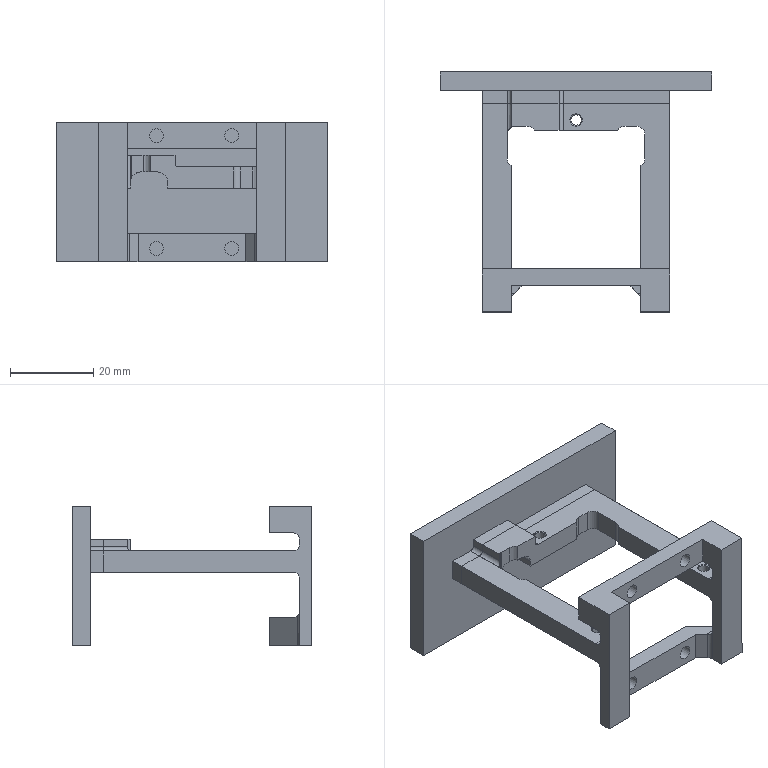NC program | NX | posted with a generic post | part box 65 x 57.5 x 33.5 mm
Whole program:
N10 G17 G21 G94 G90
(PLANAR_PROFILING , TOOL : D8-25-D8-60-3T-ROUGH)
N12 T02 M6
N14 G54
N16 G17 G0 G90 X-10. Y-1.1 B0. C0. S4500 M3
N18 G43 Z37. H2
N20 Z8.507 B-180.
N22 G94 G1 Z6.507 F1500.
N24 X0.
N26 X45.
N28 X55.
N30 Z8.507
N32 G0 Z8.014
N34 G1 Z6.014
N36 X45.
N38 X0.
N40 X-10.
N42 Z8.014
N44 G0 Z7.521
N46 G1 Z5.521
N48 X0.
N50 X45.
N52 X55.
N54 Z7.521
N56 G0 Z7.029
N58 G1 Z5.029
N60 X45.
N62 X0.
N64 X-10.
N66 Z7.029
N68 G0 Z6.536
N70 G1 Z4.536
N72 X0.
N74 X45.
N76 X55.
N78 Z6.536
N80 G0 Z6.043
N82 G1 Z4.043
N84 X45.
N86 X0.
N88 X-10.
N90 Z6.043
N92 G0 Z5.55
N94 G1 Z3.55
N96 X0.
N98 X45.
N100 X55.
N102 Z5.55
N104 G0 Z5.057
N106 G1 Z3.057
N108 X45.
N110 X0.
N112 X-10.
N114 Z5.057
N116 G0 Z4.564
N118 G1 Z2.564
N120 X0.
N122 X45.
N124 X55.
N126 Z4.564
N128 G0 Z4.071
N130 G1 Z2.071
N132 X45.
N134 X0.
N136 X-10.
N138 Z4.071
N140 G0 Z3.579
N142 G1 Z1.579
N144 X0.
N146 X45.
N148 X55.
N150 Z3.579
N152 G0 Z3.086
N154 G1 Z1.086
N156 X45.
N158 X0.
N160 X-10.
N162 Z3.086
N164 G0 Z2.593
N166 G1 Z0.593
N168 X0.
N170 X45.
N172 X55.
N174 Z2.593
N176 G0 Z2.1
N178 G1 Z0.1
N180 X45.
N182 X0.
N184 X-10.
N186 Z2.1
N188 G0 Z37.
N190 M5
(PLANAR_PROFILING_COPY , TOOL : D8-25-D8-60-3T-FINISH)
N192 T03 M6
N194 G54
N196 G17 G0 G90 X-10. Y-1.1 B0. C0. S4500 M3
N198 G43 Z37. H3
N200 Z2. B-180.
N202 G94 G1 Z0. F1000.
N204 X0.
N206 X45.
N208 X55.
N210 Z2.
N212 G0 Z37.
N214 M5
(PLANAR_PROFILING_1 , TOOL : D3-9-D4-50-3T-ROUGH)
N216 T05 M6
N218 G54
N220 G17 G0 G90 X23.07 Y5.785 B0. C0. S4500 M3
N222 G43 Z30. H5
N224 Z2.708 B-180.
N226 G94 G1 Z-0.292 F1500.
N228 Y3.1
N230 G3 X24.57 Y1.6 R1.5
N232 G1 X24.97
N234 Y2.8
N236 G2 X26.57 Y4.4 R1.6
N238 G1 X38.
N240 G2 X39.6 Y2.8 R1.6
N242 G1 Y1.6
N244 X40.
N246 G3 X41.5 Y3.1 R1.5
N248 G1 Y5.785
N250 Z2.708
N252 G0 Z2.417
N254 G1 Z-0.583
N256 Y3.1
N258 G2 X40. Y1.6 R1.5
N260 G1 X39.6
N262 Y2.8
N264 G3 X38. Y4.4 R1.6
N266 G1 X26.57
N268 G3 X24.97 Y2.8 R1.6
N270 G1 Y1.6
N272 X24.57
N274 G2 X23.07 Y3.1 R1.5
N276 G1 Y5.785
N278 Z2.417
N280 G0 Z2.125
N282 G1 Z-0.875
N284 Y3.1
N286 G3 X24.57 Y1.6 R1.5
N288 G1 X24.97
N290 Y2.8
N292 G2 X26.57 Y4.4 R1.6
N294 G1 X38.
N296 G2 X39.6 Y2.8 R1.6
N298 G1 Y1.6
N300 X40.
N302 G3 X41.5 Y3.1 R1.5
N304 G1 Y5.785
N306 Z2.125
N308 G0 Z1.833
N310 G1 Z-1.167
N312 Y3.1
N314 G2 X40. Y1.6 R1.5
N316 G1 X39.6
N318 Y2.8
N320 G3 X38. Y4.4 R1.6
N322 G1 X26.57
N324 G3 X24.97 Y2.8 R1.6
N326 G1 Y1.6
N328 X24.57
N330 G2 X23.07 Y3.1 R1.5
N332 G1 Y5.785
N334 Z1.833
N336 G0 Z1.542
N338 G1 Z-1.458
N340 Y3.1
N342 G3 X24.57 Y1.6 R1.5
N344 G1 X24.97
N346 Y2.8
N348 G2 X26.57 Y4.4 R1.6
N350 G1 X38.
N352 G2 X39.6 Y2.8 R1.6
N354 G1 Y1.6
N356 X40.
N358 G3 X41.5 Y3.1 R1.5
N360 G1 Y5.785
N362 Z1.542
N364 G0 Z1.25
N366 G1 Z-1.75
N368 Y3.1
N370 G2 X40. Y1.6 R1.5
N372 G1 X39.6
N374 Y2.8
N376 G3 X38. Y4.4 R1.6
N378 G1 X26.57
N380 G3 X24.97 Y2.8 R1.6
N382 G1 Y1.6
N384 X24.57
N386 G2 X23.07 Y3.1 R1.5
N388 G1 Y5.785
N390 Z1.25
N392 G0 Z0.958
N394 G1 Z-2.042
N396 Y3.1
N398 G3 X24.57 Y1.6 R1.5
N400 G1 X24.97
N402 Y2.8
N404 G2 X26.57 Y4.4 R1.6
N406 G1 X38.
N408 G2 X39.6 Y2.8 R1.6
N410 G1 Y1.6
N412 X40.
N414 G3 X41.5 Y3.1 R1.5
N416 G1 Y5.785
N418 Z0.958
N420 G0 Z0.667
N422 G1 Z-2.333
N424 Y3.1
N426 G2 X40. Y1.6 R1.5
N428 G1 X39.6
N430 Y2.8
N432 G3 X38. Y4.4 R1.6
N434 G1 X26.57
N436 G3 X24.97 Y2.8 R1.6
N438 G1 Y1.6
N440 X24.57
N442 G2 X23.07 Y3.1 R1.5
N444 G1 Y5.785
N446 Z0.667
N448 G0 Z0.375
N450 G1 Z-2.625
N452 Y3.1
N454 G3 X24.57 Y1.6 R1.5
N456 G1 X24.97
N458 Y2.8
N460 G2 X26.57 Y4.4 R1.6
N462 G1 X38.
N464 G2 X39.6 Y2.8 R1.6
N466 G1 Y1.6
N468 X40.
N470 G3 X41.5 Y3.1 R1.5
N472 G1 Y5.785
N474 Z0.375
N476 G0 Z0.083
N478 G1 Z-2.917
N480 Y3.1
N482 G2 X40. Y1.6 R1.5
N484 G1 X39.6
N486 Y2.8
N488 G3 X38. Y4.4 R1.6
N490 G1 X26.57
N492 G3 X24.97 Y2.8 R1.6
N494 G1 Y1.6
N496 X24.57
N498 G2 X23.07 Y3.1 R1.5
N500 G1 Y5.785
N502 Z0.083
N504 G0 Z-0.208
N506 G1 Z-3.208
N508 Y3.1
N510 G3 X24.57 Y1.6 R1.5
N512 G1 X24.97
N514 Y2.8
N516 G2 X26.57 Y4.4 R1.6
N518 G1 X38.
N520 G2 X39.6 Y2.8 R1.6
N522 G1 Y1.6
N524 X40.
N526 G3 X41.5 Y3.1 R1.5
N528 G1 Y5.785
N530 Z-0.208
N532 G0 Z-0.5
N534 G1 Z-3.5
N536 Y3.1
N538 G2 X40. Y1.6 R1.5
N540 G1 X39.6
N542 Y2.8
N544 G3 X38. Y4.4 R1.6
N546 G1 X26.57
N548 G3 X24.97 Y2.8 R1.6
N550 G1 Y1.6
N552 X24.57
N554 G2 X23.07 Y3.1 R1.5
N556 G1 Y5.785
N558 Z-0.5
N560 G0 Z-0.792
N562 G1 Z-3.792
N564 Y3.1
N566 G3 X24.57 Y1.6 R1.5
N568 G1 X24.97
N570 Y2.8
N572 G2 X26.57 Y4.4 R1.6
N574 G1 X38.
N576 G2 X39.6 Y2.8 R1.6
N578 G1 Y1.6
N580 X40.
N582 G3 X41.5 Y3.1 R1.5
N584 G1 Y5.785
N586 Z-0.792
N588 G0 Z-1.083
N590 G1 Z-4.083
N592 Y3.1
N594 G2 X40. Y1.6 R1.5
N596 G1 X39.6
N598 Y2.8
N600 G3 X38. Y4.4 R1.6
N602 G1 X26.57
N604 G3 X24.97 Y2.8 R1.6
N606 G1 Y1.6
N608 X24.57
N610 G2 X23.07 Y3.1 R1.5
N612 G1 Y5.785
N614 Z-1.083
N616 G0 Z-1.375
N618 G1 Z-4.375
N620 Y3.1
N622 G3 X24.57 Y1.6 R1.5
N624 G1 X24.97
N626 Y2.8
N628 G2 X26.57 Y4.4 R1.6
N630 G1 X38.
N632 G2 X39.6 Y2.8 R1.6
N634 G1 Y1.6
N636 X40.
N638 G3 X41.5 Y3.1 R1.5
N640 G1 Y5.785
N642 Z-1.375
N644 G0 Z-1.667
N646 G1 Z-4.667
N648 Y3.1
N650 G2 X40. Y1.6 R1.5
N652 G1 X39.6
N654 Y2.8
N656 G3 X38. Y4.4 R1.6
N658 G1 X26.57
N660 G3 X24.97 Y2.8 R1.6
N662 G1 Y1.6
N664 X24.57
N666 G2 X23.07 Y3.1 R1.5
N668 G1 Y5.785
N670 Z-1.667
N672 G0 Z-1.958
N674 G1 Z-4.958
N676 Y3.1
N678 G3 X24.57 Y1.6 R1.5
N680 G1 X24.97
N682 Y2.8
N684 G2 X26.57 Y4.4 R1.6
N686 G1 X38.
N688 G2 X39.6 Y2.8 R1.6
N690 G1 Y1.6
N692 X40.
N694 G3 X41.5 Y3.1 R1.5
N696 G1 Y5.785
N698 Z-1.958
N700 G0 Z-2.25
N702 G1 Z-5.25
N704 Y3.1
N706 G2 X40. Y1.6 R1.5
N708 G1 X39.6
N710 Y2.8
N712 G3 X38. Y4.4 R1.6
N714 G1 X26.57
N716 G3 X24.97 Y2.8 R1.6
N718 G1 Y1.6
N720 X24.57
N722 G2 X23.07 Y3.1 R1.5
N724 G1 Y5.785
N726 Z-2.25
N728 G0 Z-2.542
N730 G1 Z-5.542
N732 Y3.1
N734 G3 X24.57 Y1.6 R1.5
N736 G1 X24.97
N738 Y2.8
N740 G2 X26.57 Y4.4 R1.6
N742 G1 X38.
N744 G2 X39.6 Y2.8 R1.6
N746 G1 Y1.6
N748 X40.
N750 G3 X41.5 Y3.1 R1.5
N752 G1 Y5.785
N754 Z-2.542
N756 G0 Z-2.833
N758 G1 Z-5.833
N760 Y3.1
N762 G2 X40. Y1.6 R1.5
N764 G1 X39.6
N766 Y2.8
N768 G3 X38. Y4.4 R1.6
N770 G1 X26.57
N772 G3 X24.97 Y2.8 R1.6
N774 G1 Y1.6
N776 X24.57
N778 G2 X23.07 Y3.1 R1.5
N780 G1 Y5.785
N782 Z-2.833
N784 G0 Z-3.125
N786 G1 Z-6.125
N788 Y3.1
N790 G3 X24.57 Y1.6 R1.5
N792 G1 X24.97
N794 Y2.8
N796 G2 X26.57 Y4.4 R1.6
N798 G1 X38.
N800 G2 X39.6 Y2.8 R1.6
N802 G1 Y1.6
N804 X40.
N806 G3 X41.5 Y3.1 R1.5
N808 G1 Y5.785
N810 Z-3.125
N812 G0 Z-3.417
N814 G1 Z-6.417
N816 Y3.1
N818 G2 X40. Y1.6 R1.5
N820 G1 X39.6
N822 Y2.8
N824 G3 X38. Y4.4 R1.6
N826 G1 X26.57
N828 G3 X24.97 Y2.8 R1.6
N830 G1 Y1.6
N832 X24.57
N834 G2 X23.07 Y3.1 R1.5
N836 G1 Y5.785
N838 Z-3.417
N840 G0 Z-3.708
N842 G1 Z-6.708
N844 Y3.1
N846 G3 X24.57 Y1.6 R1.5
N848 G1 X24.97
N850 Y2.8
N852 G2 X26.57 Y4.4 R1.6
N854 G1 X38.
N856 G2 X39.6 Y2.8 R1.6
N858 G1 Y1.6
N860 X40.
N862 G3 X41.5 Y3.1 R1.5
N864 G1 Y5.785
N866 Z-3.708
N868 G0 Z-4.
N870 G1 Z-7.
N872 Y3.1
N874 G2 X40. Y1.6 R1.5
N876 G1 X39.6
N878 Y2.8
N880 G3 X38. Y4.4 R1.6
N882 G1 X26.57
N884 G3 X24.97 Y2.8 R1.6
N886 G1 Y1.6
N888 X24.57
N890 G2 X23.07 Y3.1 R1.5
N892 G1 Y5.785
N894 Z-4.
N896 G0 Z30.
(PLANAR_PROFILING_1_COPY , TOOL : D3-9-D4-50-3T-ROUGH)
N898 X33.67 Y-7.1
N900 Z1.708
N902 G1 Z-0.292
N904 G3 X35.67 Y-5.1 R2.
N906 G1 Y-3.7
N908 G3 X34.77 Y-2.8 R0.9
N910 G1 X30.77
N912 G3 X29.87 Y-3.7 R0.9
N914 G1 Y-5.1
N916 G3 X31.87 Y-7.1 R2.
N918 G1 Z1.708
N920 G0 Z1.417
N922 G1 Z-0.583
N924 G2 X29.87 Y-5.1 R2.
N926 G1 Y-3.7
N928 G2 X30.77 Y-2.8 R0.9
N930 G1 X34.77
N932 G2 X35.67 Y-3.7 R0.9
N934 G1 Y-5.1
N936 G2 X33.67 Y-7.1 R2.
N938 G1 Z1.417
N940 G0 Z1.125
N942 G1 Z-0.875
N944 G3 X35.67 Y-5.1 R2.
N946 G1 Y-3.7
N948 G3 X34.77 Y-2.8 R0.9
N950 G1 X30.77
N952 G3 X29.87 Y-3.7 R0.9
N954 G1 Y-5.1
N956 G3 X31.87 Y-7.1 R2.
N958 G1 Z1.125
N960 G0 Z0.833
N962 G1 Z-1.167
N964 G2 X29.87 Y-5.1 R2.
N966 G1 Y-3.7
N968 G2 X30.77 Y-2.8 R0.9
N970 G1 X34.77
N972 G2 X35.67 Y-3.7 R0.9
N974 G1 Y-5.1
N976 G2 X33.67 Y-7.1 R2.
N978 G1 Z0.833
N980 G0 Z0.542
N982 G1 Z-1.458
N984 G3 X35.67 Y-5.1 R2.
N986 G1 Y-3.7
N988 G3 X34.77 Y-2.8 R0.9
N990 G1 X30.77
N992 G3 X29.87 Y-3.7 R0.9
N994 G1 Y-5.1
N996 G3 X31.87 Y-7.1 R2.
N998 G1 Z0.542
N1000 G0 Z0.25
N1002 G1 Z-1.75
N1004 G2 X29.87 Y-5.1 R2.
N1006 G1 Y-3.7
N1008 G2 X30.77 Y-2.8 R0.9
N1010 G1 X34.77
N1012 G2 X35.67 Y-3.7 R0.9
N1014 G1 Y-5.1
N1016 G2 X33.67 Y-7.1 R2.
N1018 G1 Z0.25
N1020 G0 Z-0.042
N1022 G1 Z-2.042
N1024 G3 X35.67 Y-5.1 R2.
N1026 G1 Y-3.7
N1028 G3 X34.77 Y-2.8 R0.9
N1030 G1 X30.77
N1032 G3 X29.87 Y-3.7 R0.9
N1034 G1 Y-5.1
N1036 G3 X31.87 Y-7.1 R2.
N1038 G1 Z-0.042
N1040 G0 Z-0.333
N1042 G1 Z-2.333
N1044 G2 X29.87 Y-5.1 R2.
N1046 G1 Y-3.7
N1048 G2 X30.77 Y-2.8 R0.9
N1050 G1 X34.77
N1052 G2 X35.67 Y-3.7 R0.9
N1054 G1 Y-5.1
N1056 G2 X33.67 Y-7.1 R2.
N1058 G1 Z-0.333
N1060 G0 Z-0.625
N1062 G1 Z-2.625
N1064 G3 X35.67 Y-5.1 R2.
N1066 G1 Y-3.7
N1068 G3 X34.77 Y-2.8 R0.9
N1070 G1 X30.77
N1072 G3 X29.87 Y-3.7 R0.9
N1074 G1 Y-5.1
N1076 G3 X31.87 Y-7.1 R2.
N1078 G1 Z-0.625
N1080 G0 Z-0.917
N1082 G1 Z-2.917
N1084 G2 X29.87 Y-5.1 R2.
N1086 G1 Y-3.7
N1088 G2 X30.77 Y-2.8 R0.9
N1090 G1 X34.77
N1092 G2 X35.67 Y-3.7 R0.9
N1094 G1 Y-5.1
N1096 G2 X33.67 Y-7.1 R2.
N1098 G1 Z-0.917
N1100 G0 Z-1.208
N1102 G1 Z-3.208
N1104 G3 X35.67 Y-5.1 R2.
N1106 G1 Y-3.7
N1108 G3 X34.77 Y-2.8 R0.9
N1110 G1 X30.77
N1112 G3 X29.87 Y-3.7 R0.9
N1114 G1 Y-5.1
N1116 G3 X31.87 Y-7.1 R2.
N1118 G1 Z-1.208
N1120 G0 Z-1.5
N1122 G1 Z-3.5
N1124 G2 X29.87 Y-5.1 R2.
N1126 G1 Y-3.7
N1128 G2 X30.77 Y-2.8 R0.9
N1130 G1 X34.77
N1132 G2 X35.67 Y-3.7 R0.9
N1134 G1 Y-5.1
N1136 G2 X33.67 Y-7.1 R2.
N1138 G1 Z-1.5
N1140 G0 Z-1.792
N1142 G1 Z-3.792
N1144 G3 X35.67 Y-5.1 R2.
N1146 G1 Y-3.7
N1148 G3 X34.77 Y-2.8 R0.9
N1150 G1 X30.77
N1152 G3 X29.87 Y-3.7 R0.9
N1154 G1 Y-5.1
N1156 G3 X31.87 Y-7.1 R2.
N1158 G1 Z-1.792
N1160 G0 Z-2.083
N1162 G1 Z-4.083
N1164 G2 X29.87 Y-5.1 R2.
N1166 G1 Y-3.7
N1168 G2 X30.77 Y-2.8 R0.9
N1170 G1 X34.77
N1172 G2 X35.67 Y-3.7 R0.9
N1174 G1 Y-5.1
N1176 G2 X33.67 Y-7.1 R2.
N1178 G1 Z-2.083
N1180 G0 Z-2.375
N1182 G1 Z-4.375
N1184 G3 X35.67 Y-5.1 R2.
N1186 G1 Y-3.7
N1188 G3 X34.77 Y-2.8 R0.9
N1190 G1 X30.77
N1192 G3 X29.87 Y-3.7 R0.9
N1194 G1 Y-5.1
N1196 G3 X31.87 Y-7.1 R2.
N1198 G1 Z-2.375
N1200 G0 Z-2.667
N1202 G1 Z-4.667
N1204 G2 X29.87 Y-5.1 R2.
N1206 G1 Y-3.7
N1208 G2 X30.77 Y-2.8 R0.9
N1210 G1 X34.77
N1212 G2 X35.67 Y-3.7 R0.9
N1214 G1 Y-5.1
N1216 G2 X33.67 Y-7.1 R2.
N1218 G1 Z-2.667
N1220 G0 Z-2.958
N1222 G1 Z-4.958
N1224 G3 X35.67 Y-5.1 R2.
N1226 G1 Y-3.7
N1228 G3 X34.77 Y-2.8 R0.9
N1230 G1 X30.77
N1232 G3 X29.87 Y-3.7 R0.9
N1234 G1 Y-5.1
N1236 G3 X31.87 Y-7.1 R2.
N1238 G1 Z-2.958
N1240 G0 Z-3.25
N1242 G1 Z-5.25
N1244 G2 X29.87 Y-5.1 R2.
N1246 G1 Y-3.7
N1248 G2 X30.77 Y-2.8 R0.9
N1250 G1 X34.77
N1252 G2 X35.67 Y-3.7 R0.9
N1254 G1 Y-5.1
N1256 G2 X33.67 Y-7.1 R2.
N1258 G1 Z-3.25
N1260 G0 Z-3.542
N1262 G1 Z-5.542
N1264 G3 X35.67 Y-5.1 R2.
N1266 G1 Y-3.7
N1268 G3 X34.77 Y-2.8 R0.9
N1270 G1 X30.77
N1272 G3 X29.87 Y-3.7 R0.9
N1274 G1 Y-5.1
N1276 G3 X31.87 Y-7.1 R2.
N1278 G1 Z-3.542
N1280 G0 Z-3.833
N1282 G1 Z-5.833
N1284 G2 X29.87 Y-5.1 R2.
N1286 G1 Y-3.7
N1288 G2 X30.77 Y-2.8 R0.9
N1290 G1 X34.77
N1292 G2 X35.67 Y-3.7 R0.9
N1294 G1 Y-5.1
N1296 G2 X33.67 Y-7.1 R2.
N1298 G1 Z-3.833
N1300 G0 Z-4.125
N1302 G1 Z-6.125
N1304 G3 X35.67 Y-5.1 R2.
N1306 G1 Y-3.7
N1308 G3 X34.77 Y-2.8 R0.9
N1310 G1 X30.77
N1312 G3 X29.87 Y-3.7 R0.9
N1314 G1 Y-5.1
N1316 G3 X31.87 Y-7.1 R2.
N1318 G1 Z-4.125
N1320 G0 Z-4.417
N1322 G1 Z-6.417
N1324 G2 X29.87 Y-5.1 R2.
N1326 G1 Y-3.7
N1328 G2 X30.77 Y-2.8 R0.9
N1330 G1 X34.77
N1332 G2 X35.67 Y-3.7 R0.9
N1334 G1 Y-5.1
N1336 G2 X33.67 Y-7.1 R2.
N1338 G1 Z-4.417
N1340 G0 Z-4.708
N1342 G1 Z-6.708
N1344 G3 X35.67 Y-5.1 R2.
N1346 G1 Y-3.7
N1348 G3 X34.77 Y-2.8 R0.9
N1350 G1 X30.77
N1352 G3 X29.87 Y-3.7 R0.9
N1354 G1 Y-5.1
N1356 G3 X31.87 Y-7.1 R2.
N1358 G1 Z-4.708
N1360 G0 Z-5.
N1362 G1 Z-7.
N1364 G2 X29.87 Y-5.1 R2.
N1366 G1 Y-3.7
N1368 G2 X30.77 Y-2.8 R0.9
N1370 G1 X34.77
N1372 G2 X35.67 Y-3.7 R0.9
N1374 G1 Y-5.1
N1376 G2 X33.67 Y-7.1 R2.
N1378 G1 Z-5.
N1380 G0 Z30.
N1382 M5
(PLANAR_PROFILING_1_COPY_1 , TOOL : D3-9-D4-50-3T-FINISH)
N1384 T06 M6
N1386 G54
N1388 G17 G0 G90 X23.07 Y5.628 B0. C0. S4500 M3
N1390 G43 Z30. H6
N1392 Z-4. B-180.
N1394 G94 G1 Z-7. F800.
N1396 Y3.
N1398 G3 X24.57 Y1.5 R1.5
N1400 G1 X25.07
N1402 Y2.8
N1404 G2 X26.57 Y4.3 R1.5
N1406 G1 X38.
N1408 G2 X39.5 Y2.8 R1.5
N1410 G1 Y1.5
N1412 X40.
N1414 G3 X41.5 Y3. R1.5
N1416 G1 Y5.628
N1418 Z-4.
N1420 G0 Z30.
(PLANAR_PROFILING_1_COPY_COPY , TOOL : D3-9-D4-50-3T-FINISH)
N1422 X33.77 Y-7.1
N1424 Z-5.
N1426 G1 Z-7.
N1428 G3 X35.77 Y-5.1 R2.
N1430 G1 Y-3.7
N1432 G3 X34.77 Y-2.7 R1.
N1434 G1 X30.77
N1436 G3 X29.77 Y-3.7 R1.
N1438 G1 Y-5.1
N1440 G3 X31.77 Y-7.1 R2.
N1442 G1 Z-5.
N1444 G0 Z30.
N1446 M5
(平面铣倒角_1 , TOOL : 倒角D4-90度)
N1448 T08 M6
N1450 G54
N1452 G17 G0 G90 X14.754 Y-6.264 B0. C0. S3500 M3
N1454 G43 Z30. H8
N1456 Z2. B-180.
N1458 G94 G1 Z-1. F1000.
N1460 G41 X14.275 Y-6.12 D8
N1462 X14.135 Y-6.1
N1464 X0.
N1466 G2 X-1. Y-5.1 R1.
N1468 G1 Y0.
N1470 G2 X0. Y1. R1.
N1472 G1 X25.57
N1474 Y2.8
N1476 G2 X26.57 Y3.8 R1.
N1478 G1 X38.
N1480 G2 X39. Y2.8 R1.
N1482 G1 Y1.
N1484 X45.
N1486 G2 X46. Y0. R1.
N1488 G1 Y-5.1
N1490 G2 X45. Y-6.1 R1.
N1492 G1 X37.27
N1494 G2 X36.27 Y-5.1 R1.
N1496 G1 Y-3.7
N1498 G3 X34.77 Y-2.2 R1.5
N1500 G1 X30.77
N1502 G3 X29.27 Y-3.7 R1.5
N1504 G1 Y-5.1
N1506 G2 X28.27 Y-6.1 R1.
N1508 G1 X14.135
N1510 X13.995 Y-6.12
N1512 G40
N1514 X13.516 Y-6.264
N1516 Z2.
N1518 G0 Z30.
N1520 M5
(PLANAR_PROFILING_1_COPY_1_COPY , TOOL : D2-6-D4-50-3T-FINISH)
N1522 T13 M6
N1524 G54
N1526 G17 G0 G90 X23.57 Y5.446 B0. C0. S4500 M3
N1528 G43 Z30. H13
N1530 Z0.667 B-180.
N1532 G94 G1 Z-2.333 F800.
N1534 Y2.
N1536 G3 X24.57 Y1. R1.
N1538 G1 X25.57
N1540 Y2.8
N1542 G2 X26.57 Y3.8 R1.
N1544 G1 X38.
N1546 G2 X39. Y2.8 R1.
N1548 G1 Y1.
N1550 X40.
N1552 G3 X41. Y2. R1.
N1554 G1 Y5.446
N1556 Z0.667
N1558 G0 Z-1.667
N1560 G1 Z-4.667
N1562 Y2.
N1564 G2 X40. Y1. R1.
N1566 G1 X39.
N1568 Y2.8
N1570 G3 X38. Y3.8 R1.
N1572 G1 X26.57
N1574 G3 X25.57 Y2.8 R1.
N1576 G1 Y1.
N1578 X24.57
N1580 G2 X23.57 Y2. R1.
N1582 G1 Y5.446
N1584 Z-1.667
N1586 G0 Z-4.
N1588 G1 Z-7.
N1590 Y2.
N1592 G3 X24.57 Y1. R1.
N1594 G1 X25.57
N1596 Y2.8
N1598 G2 X26.57 Y3.8 R1.
N1600 G1 X38.
N1602 G2 X39. Y2.8 R1.
N1604 G1 Y1.
N1606 X40.
N1608 G3 X41. Y2. R1.
N1610 G1 Y5.446
N1612 Z-4.
N1614 G0 Z30.
N1616 M5
N1618 M2